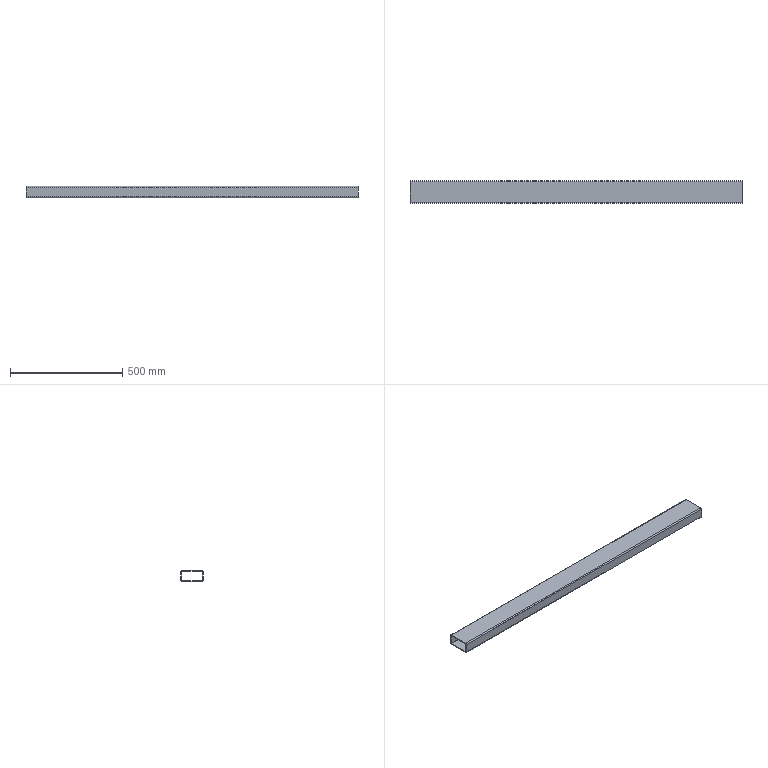Part | SolidWorks | features BaseBody 1 | 1 solid | 18 faces | box 1480 x 100 x 50 mm | volume 1650789 mm3 | plane 10 | cylinder 8 | commonest cylinder face diameters 2 x4 10 x4
STEP:
#1=CARTESIAN_POINT('',(-740.,45.,-25.));
#2=VERTEX_POINT('',#1);
#3=CARTESIAN_POINT('',(-740.,50.,-20.));
#4=VERTEX_POINT('',#3);
#5=CARTESIAN_POINT('',(-740.,45.,-20.));
#6=DIRECTION('',(1.,0.,0.));
#7=DIRECTION('',(0.,0.,-1.));
#8=AXIS2_PLACEMENT_3D('',#5,#6,#7);
#9=CIRCLE('',#8,5.);
#10=EDGE_CURVE('',#2,#4,#9,.T.);
#11=ORIENTED_EDGE('',*,*,#10,.T.);
#12=CARTESIAN_POINT('',(740.,50.,-20.));
#13=VERTEX_POINT('',#12);
#14=CARTESIAN_POINT('',(740.,50.,-20.));
#15=DIRECTION('',(-1.,0.,0.));
#16=VECTOR('',#15,1000.);
#17=LINE('',#14,#16);
#18=EDGE_CURVE('',#13,#4,#17,.T.);
#19=ORIENTED_EDGE('',*,*,#18,.F.);
#20=CARTESIAN_POINT('',(740.,45.,-25.));
#21=VERTEX_POINT('',#20);
#22=CARTESIAN_POINT('',(740.,45.,-20.));
#23=DIRECTION('',(1.,0.,0.));
#24=DIRECTION('',(0.,0.,-1.));
#25=AXIS2_PLACEMENT_3D('',#22,#23,#24);
#26=CIRCLE('',#25,5.);
#27=EDGE_CURVE('',#21,#13,#26,.T.);
#28=ORIENTED_EDGE('',*,*,#27,.F.);
#29=CARTESIAN_POINT('',(740.,45.,-25.));
#30=DIRECTION('',(-1.,0.,0.));
#31=VECTOR('',#30,1000.);
#32=LINE('',#29,#31);
#33=EDGE_CURVE('',#21,#2,#32,.T.);
#34=ORIENTED_EDGE('',*,*,#33,.T.);
#35=EDGE_LOOP('',(#11,#19,#28,#34));
#36=FACE_OUTER_BOUND('',#35,.T.);
#37=CARTESIAN_POINT('',(740.,45.,-20.));
#38=DIRECTION('',(-1.,0.,0.));
#39=DIRECTION('',(0.,0.,1.));
#40=AXIS2_PLACEMENT_3D('',#37,#38,#39);
#41=CYLINDRICAL_SURFACE('',#40,5.);
#42=ADVANCED_FACE('',(#36),#41,.T.);
#43=CARTESIAN_POINT('',(-740.,50.,20.));
#44=VERTEX_POINT('',#43);
#45=CARTESIAN_POINT('',(-740.,50.,-20.));
#46=DIRECTION('',(0.,0.,1.));
#47=VECTOR('',#46,1000.);
#48=LINE('',#45,#47);
#49=EDGE_CURVE('',#4,#44,#48,.T.);
#50=ORIENTED_EDGE('',*,*,#49,.T.);
#51=CARTESIAN_POINT('',(740.,50.,20.));
#52=VERTEX_POINT('',#51);
#53=CARTESIAN_POINT('',(740.,50.,20.));
#54=DIRECTION('',(-1.,0.,0.));
#55=VECTOR('',#54,1000.);
#56=LINE('',#53,#55);
#57=EDGE_CURVE('',#52,#44,#56,.T.);
#58=ORIENTED_EDGE('',*,*,#57,.F.);
#59=CARTESIAN_POINT('',(740.,50.,-20.));
#60=DIRECTION('',(0.,0.,1.));
#61=VECTOR('',#60,1000.);
#62=LINE('',#59,#61);
#63=EDGE_CURVE('',#13,#52,#62,.T.);
#64=ORIENTED_EDGE('',*,*,#63,.F.);
#65=ORIENTED_EDGE('',*,*,#18,.T.);
#66=EDGE_LOOP('',(#50,#58,#64,#65));
#67=FACE_OUTER_BOUND('',#66,.T.);
#68=CARTESIAN_POINT('',(740.,50.,-20.));
#69=DIRECTION('',(0.,-1.,0.));
#70=DIRECTION('',(0.,0.,-1.));
#71=AXIS2_PLACEMENT_3D('',#68,#69,#70);
#72=PLANE('',#71);
#73=ADVANCED_FACE('',(#67),#72,.F.);
#74=CARTESIAN_POINT('',(-740.,45.,25.));
#75=VERTEX_POINT('',#74);
#76=CARTESIAN_POINT('',(-740.,45.,20.));
#77=DIRECTION('',(1.,0.,0.));
#78=DIRECTION('',(0.,0.,-1.));
#79=AXIS2_PLACEMENT_3D('',#76,#77,#78);
#80=CIRCLE('',#79,5.);
#81=EDGE_CURVE('',#44,#75,#80,.T.);
#82=ORIENTED_EDGE('',*,*,#81,.T.);
#83=CARTESIAN_POINT('',(740.,45.,25.));
#84=VERTEX_POINT('',#83);
#85=CARTESIAN_POINT('',(740.,45.,25.));
#86=DIRECTION('',(-1.,0.,0.));
#87=VECTOR('',#86,1000.);
#88=LINE('',#85,#87);
#89=EDGE_CURVE('',#84,#75,#88,.T.);
#90=ORIENTED_EDGE('',*,*,#89,.F.);
#91=CARTESIAN_POINT('',(740.,45.,20.));
#92=DIRECTION('',(1.,0.,0.));
#93=DIRECTION('',(0.,0.,-1.));
#94=AXIS2_PLACEMENT_3D('',#91,#92,#93);
#95=CIRCLE('',#94,5.);
#96=EDGE_CURVE('',#52,#84,#95,.T.);
#97=ORIENTED_EDGE('',*,*,#96,.F.);
#98=ORIENTED_EDGE('',*,*,#57,.T.);
#99=EDGE_LOOP('',(#82,#90,#97,#98));
#100=FACE_OUTER_BOUND('',#99,.T.);
#101=CARTESIAN_POINT('',(740.,45.,20.));
#102=DIRECTION('',(-1.,0.,0.));
#103=DIRECTION('',(0.,0.,1.));
#104=AXIS2_PLACEMENT_3D('',#101,#102,#103);
#105=CYLINDRICAL_SURFACE('',#104,5.);
#106=ADVANCED_FACE('',(#100),#105,.T.);
#107=CARTESIAN_POINT('',(-740.,-45.,25.));
#108=VERTEX_POINT('',#107);
#109=CARTESIAN_POINT('',(-740.,-45.,25.));
#110=DIRECTION('',(0.,-1.,0.));
#111=VECTOR('',#110,1000.);
#112=LINE('',#109,#111);
#113=EDGE_CURVE('',#75,#108,#112,.T.);
#114=ORIENTED_EDGE('',*,*,#113,.T.);
#115=CARTESIAN_POINT('',(740.,-45.,25.));
#116=VERTEX_POINT('',#115);
#117=CARTESIAN_POINT('',(740.,-45.,25.));
#118=DIRECTION('',(-1.,0.,0.));
#119=VECTOR('',#118,1000.);
#120=LINE('',#117,#119);
#121=EDGE_CURVE('',#116,#108,#120,.T.);
#122=ORIENTED_EDGE('',*,*,#121,.F.);
#123=CARTESIAN_POINT('',(740.,-45.,25.));
#124=DIRECTION('',(0.,-1.,0.));
#125=VECTOR('',#124,1000.);
#126=LINE('',#123,#125);
#127=EDGE_CURVE('',#84,#116,#126,.T.);
#128=ORIENTED_EDGE('',*,*,#127,.F.);
#129=ORIENTED_EDGE('',*,*,#89,.T.);
#130=EDGE_LOOP('',(#114,#122,#128,#129));
#131=FACE_OUTER_BOUND('',#130,.T.);
#132=CARTESIAN_POINT('',(740.,-45.,25.));
#133=DIRECTION('',(0.,0.,-1.));
#134=DIRECTION('',(0.,1.,0.));
#135=AXIS2_PLACEMENT_3D('',#132,#133,#134);
#136=PLANE('',#135);
#137=ADVANCED_FACE('',(#131),#136,.F.);
#138=CARTESIAN_POINT('',(-740.,-50.,20.));
#139=VERTEX_POINT('',#138);
#140=CARTESIAN_POINT('',(-740.,-45.,20.));
#141=DIRECTION('',(1.,0.,0.));
#142=DIRECTION('',(0.,0.,-1.));
#143=AXIS2_PLACEMENT_3D('',#140,#141,#142);
#144=CIRCLE('',#143,5.);
#145=EDGE_CURVE('',#108,#139,#144,.T.);
#146=ORIENTED_EDGE('',*,*,#145,.T.);
#147=CARTESIAN_POINT('',(740.,-50.,20.));
#148=VERTEX_POINT('',#147);
#149=CARTESIAN_POINT('',(740.,-50.,20.));
#150=DIRECTION('',(-1.,0.,0.));
#151=VECTOR('',#150,1000.);
#152=LINE('',#149,#151);
#153=EDGE_CURVE('',#148,#139,#152,.T.);
#154=ORIENTED_EDGE('',*,*,#153,.F.);
#155=CARTESIAN_POINT('',(740.,-45.,20.));
#156=DIRECTION('',(1.,0.,0.));
#157=DIRECTION('',(0.,0.,-1.));
#158=AXIS2_PLACEMENT_3D('',#155,#156,#157);
#159=CIRCLE('',#158,5.);
#160=EDGE_CURVE('',#116,#148,#159,.T.);
#161=ORIENTED_EDGE('',*,*,#160,.F.);
#162=ORIENTED_EDGE('',*,*,#121,.T.);
#163=EDGE_LOOP('',(#146,#154,#161,#162));
#164=FACE_OUTER_BOUND('',#163,.T.);
#165=CARTESIAN_POINT('',(740.,-45.,20.));
#166=DIRECTION('',(-1.,0.,0.));
#167=DIRECTION('',(0.,0.,1.));
#168=AXIS2_PLACEMENT_3D('',#165,#166,#167);
#169=CYLINDRICAL_SURFACE('',#168,5.);
#170=ADVANCED_FACE('',(#164),#169,.T.);
#171=CARTESIAN_POINT('',(-740.,-50.,-20.));
#172=VERTEX_POINT('',#171);
#173=CARTESIAN_POINT('',(-740.,-50.,20.));
#174=DIRECTION('',(0.,0.,-1.));
#175=VECTOR('',#174,1000.);
#176=LINE('',#173,#175);
#177=EDGE_CURVE('',#139,#172,#176,.T.);
#178=ORIENTED_EDGE('',*,*,#177,.T.);
#179=CARTESIAN_POINT('',(740.,-50.,-20.));
#180=VERTEX_POINT('',#179);
#181=CARTESIAN_POINT('',(740.,-50.,-20.));
#182=DIRECTION('',(-1.,0.,0.));
#183=VECTOR('',#182,1000.);
#184=LINE('',#181,#183);
#185=EDGE_CURVE('',#180,#172,#184,.T.);
#186=ORIENTED_EDGE('',*,*,#185,.F.);
#187=CARTESIAN_POINT('',(740.,-50.,20.));
#188=DIRECTION('',(0.,0.,-1.));
#189=VECTOR('',#188,1000.);
#190=LINE('',#187,#189);
#191=EDGE_CURVE('',#148,#180,#190,.T.);
#192=ORIENTED_EDGE('',*,*,#191,.F.);
#193=ORIENTED_EDGE('',*,*,#153,.T.);
#194=EDGE_LOOP('',(#178,#186,#192,#193));
#195=FACE_OUTER_BOUND('',#194,.T.);
#196=CARTESIAN_POINT('',(740.,-50.,20.));
#197=DIRECTION('',(0.,1.,0.));
#198=DIRECTION('',(0.,0.,1.));
#199=AXIS2_PLACEMENT_3D('',#196,#197,#198);
#200=PLANE('',#199);
#201=ADVANCED_FACE('',(#195),#200,.F.);
#202=CARTESIAN_POINT('',(-740.,-45.,-25.));
#203=VERTEX_POINT('',#202);
#204=CARTESIAN_POINT('',(-740.,-45.,-20.));
#205=DIRECTION('',(1.,0.,0.));
#206=DIRECTION('',(0.,0.,-1.));
#207=AXIS2_PLACEMENT_3D('',#204,#205,#206);
#208=CIRCLE('',#207,5.);
#209=EDGE_CURVE('',#172,#203,#208,.T.);
#210=ORIENTED_EDGE('',*,*,#209,.T.);
#211=CARTESIAN_POINT('',(740.,-45.,-25.));
#212=VERTEX_POINT('',#211);
#213=CARTESIAN_POINT('',(740.,-45.,-25.));
#214=DIRECTION('',(-1.,0.,0.));
#215=VECTOR('',#214,1000.);
#216=LINE('',#213,#215);
#217=EDGE_CURVE('',#212,#203,#216,.T.);
#218=ORIENTED_EDGE('',*,*,#217,.F.);
#219=CARTESIAN_POINT('',(740.,-45.,-20.));
#220=DIRECTION('',(1.,0.,0.));
#221=DIRECTION('',(0.,0.,-1.));
#222=AXIS2_PLACEMENT_3D('',#219,#220,#221);
#223=CIRCLE('',#222,5.);
#224=EDGE_CURVE('',#180,#212,#223,.T.);
#225=ORIENTED_EDGE('',*,*,#224,.F.);
#226=ORIENTED_EDGE('',*,*,#185,.T.);
#227=EDGE_LOOP('',(#210,#218,#225,#226));
#228=FACE_OUTER_BOUND('',#227,.T.);
#229=CARTESIAN_POINT('',(740.,-45.,-20.));
#230=DIRECTION('',(-1.,0.,0.));
#231=DIRECTION('',(0.,0.,1.));
#232=AXIS2_PLACEMENT_3D('',#229,#230,#231);
#233=CYLINDRICAL_SURFACE('',#232,5.);
#234=ADVANCED_FACE('',(#228),#233,.T.);
#235=CARTESIAN_POINT('',(-740.,46.,20.));
#236=VERTEX_POINT('',#235);
#237=CARTESIAN_POINT('',(-740.,45.,21.));
#238=VERTEX_POINT('',#237);
#239=CARTESIAN_POINT('',(-740.,45.,20.));
#240=DIRECTION('',(1.,0.,0.));
#241=DIRECTION('',(0.,0.,-1.));
#242=AXIS2_PLACEMENT_3D('',#239,#240,#241);
#243=CIRCLE('',#242,1.);
#244=EDGE_CURVE('',#236,#238,#243,.T.);
#245=ORIENTED_EDGE('',*,*,#244,.F.);
#246=CARTESIAN_POINT('',(740.,46.,20.));
#247=VERTEX_POINT('',#246);
#248=CARTESIAN_POINT('',(740.,46.,20.));
#249=DIRECTION('',(-1.,0.,0.));
#250=VECTOR('',#249,1000.);
#251=LINE('',#248,#250);
#252=EDGE_CURVE('',#247,#236,#251,.T.);
#253=ORIENTED_EDGE('',*,*,#252,.F.);
#254=CARTESIAN_POINT('',(740.,45.,21.));
#255=VERTEX_POINT('',#254);
#256=CARTESIAN_POINT('',(740.,45.,20.));
#257=DIRECTION('',(1.,0.,0.));
#258=DIRECTION('',(0.,0.,-1.));
#259=AXIS2_PLACEMENT_3D('',#256,#257,#258);
#260=CIRCLE('',#259,1.);
#261=EDGE_CURVE('',#247,#255,#260,.T.);
#262=ORIENTED_EDGE('',*,*,#261,.T.);
#263=CARTESIAN_POINT('',(740.,45.,21.));
#264=DIRECTION('',(-1.,0.,0.));
#265=VECTOR('',#264,1000.);
#266=LINE('',#263,#265);
#267=EDGE_CURVE('',#255,#238,#266,.T.);
#268=ORIENTED_EDGE('',*,*,#267,.T.);
#269=EDGE_LOOP('',(#245,#253,#262,#268));
#270=FACE_OUTER_BOUND('',#269,.T.);
#271=CARTESIAN_POINT('',(740.,45.,20.));
#272=DIRECTION('',(-1.,0.,0.));
#273=DIRECTION('',(0.,0.,1.));
#274=AXIS2_PLACEMENT_3D('',#271,#272,#273);
#275=CYLINDRICAL_SURFACE('',#274,1.);
#276=ADVANCED_FACE('',(#270),#275,.F.);
#277=CARTESIAN_POINT('',(-740.,46.,-20.));
#278=VERTEX_POINT('',#277);
#279=CARTESIAN_POINT('',(-740.,46.,-20.));
#280=DIRECTION('',(0.,0.,1.));
#281=VECTOR('',#280,1000.);
#282=LINE('',#279,#281);
#283=EDGE_CURVE('',#278,#236,#282,.T.);
#284=ORIENTED_EDGE('',*,*,#283,.F.);
#285=CARTESIAN_POINT('',(740.,46.,-20.));
#286=VERTEX_POINT('',#285);
#287=CARTESIAN_POINT('',(740.,46.,-20.));
#288=DIRECTION('',(-1.,0.,0.));
#289=VECTOR('',#288,1000.);
#290=LINE('',#287,#289);
#291=EDGE_CURVE('',#286,#278,#290,.T.);
#292=ORIENTED_EDGE('',*,*,#291,.F.);
#293=CARTESIAN_POINT('',(740.,46.,-20.));
#294=DIRECTION('',(0.,0.,1.));
#295=VECTOR('',#294,1000.);
#296=LINE('',#293,#295);
#297=EDGE_CURVE('',#286,#247,#296,.T.);
#298=ORIENTED_EDGE('',*,*,#297,.T.);
#299=ORIENTED_EDGE('',*,*,#252,.T.);
#300=EDGE_LOOP('',(#284,#292,#298,#299));
#301=FACE_OUTER_BOUND('',#300,.T.);
#302=CARTESIAN_POINT('',(740.,46.,-20.));
#303=DIRECTION('',(0.,-1.,0.));
#304=DIRECTION('',(0.,0.,-1.));
#305=AXIS2_PLACEMENT_3D('',#302,#303,#304);
#306=PLANE('',#305);
#307=ADVANCED_FACE('',(#301),#306,.T.);
#308=CARTESIAN_POINT('',(-740.,45.,-21.));
#309=VERTEX_POINT('',#308);
#310=CARTESIAN_POINT('',(-740.,45.,-20.));
#311=DIRECTION('',(1.,0.,0.));
#312=DIRECTION('',(0.,0.,-1.));
#313=AXIS2_PLACEMENT_3D('',#310,#311,#312);
#314=CIRCLE('',#313,1.);
#315=EDGE_CURVE('',#309,#278,#314,.T.);
#316=ORIENTED_EDGE('',*,*,#315,.F.);
#317=CARTESIAN_POINT('',(740.,45.,-21.));
#318=VERTEX_POINT('',#317);
#319=CARTESIAN_POINT('',(740.,45.,-21.));
#320=DIRECTION('',(-1.,0.,0.));
#321=VECTOR('',#320,1000.);
#322=LINE('',#319,#321);
#323=EDGE_CURVE('',#318,#309,#322,.T.);
#324=ORIENTED_EDGE('',*,*,#323,.F.);
#325=CARTESIAN_POINT('',(740.,45.,-20.));
#326=DIRECTION('',(1.,0.,0.));
#327=DIRECTION('',(0.,0.,-1.));
#328=AXIS2_PLACEMENT_3D('',#325,#326,#327);
#329=CIRCLE('',#328,1.);
#330=EDGE_CURVE('',#318,#286,#329,.T.);
#331=ORIENTED_EDGE('',*,*,#330,.T.);
#332=ORIENTED_EDGE('',*,*,#291,.T.);
#333=EDGE_LOOP('',(#316,#324,#331,#332));
#334=FACE_OUTER_BOUND('',#333,.T.);
#335=CARTESIAN_POINT('',(740.,45.,-20.));
#336=DIRECTION('',(-1.,0.,0.));
#337=DIRECTION('',(0.,0.,1.));
#338=AXIS2_PLACEMENT_3D('',#335,#336,#337);
#339=CYLINDRICAL_SURFACE('',#338,1.);
#340=ADVANCED_FACE('',(#334),#339,.F.);
#341=CARTESIAN_POINT('',(-740.,-45.,-21.));
#342=VERTEX_POINT('',#341);
#343=CARTESIAN_POINT('',(-740.,45.,-21.));
#344=DIRECTION('',(0.,1.,0.));
#345=VECTOR('',#344,1000.);
#346=LINE('',#343,#345);
#347=EDGE_CURVE('',#342,#309,#346,.T.);
#348=ORIENTED_EDGE('',*,*,#347,.F.);
#349=CARTESIAN_POINT('',(740.,-45.,-21.));
#350=VERTEX_POINT('',#349);
#351=CARTESIAN_POINT('',(740.,-45.,-21.));
#352=DIRECTION('',(-1.,0.,0.));
#353=VECTOR('',#352,1000.);
#354=LINE('',#351,#353);
#355=EDGE_CURVE('',#350,#342,#354,.T.);
#356=ORIENTED_EDGE('',*,*,#355,.F.);
#357=CARTESIAN_POINT('',(740.,45.,-21.));
#358=DIRECTION('',(0.,1.,0.));
#359=VECTOR('',#358,1000.);
#360=LINE('',#357,#359);
#361=EDGE_CURVE('',#350,#318,#360,.T.);
#362=ORIENTED_EDGE('',*,*,#361,.T.);
#363=ORIENTED_EDGE('',*,*,#323,.T.);
#364=EDGE_LOOP('',(#348,#356,#362,#363));
#365=FACE_OUTER_BOUND('',#364,.T.);
#366=CARTESIAN_POINT('',(740.,45.,-21.));
#367=DIRECTION('',(0.,0.,1.));
#368=DIRECTION('',(1.,0.,0.));
#369=AXIS2_PLACEMENT_3D('',#366,#367,#368);
#370=PLANE('',#369);
#371=ADVANCED_FACE('',(#365),#370,.T.);
#372=CARTESIAN_POINT('',(-740.,-46.,-20.));
#373=VERTEX_POINT('',#372);
#374=CARTESIAN_POINT('',(-740.,-45.,-20.));
#375=DIRECTION('',(1.,0.,0.));
#376=DIRECTION('',(0.,0.,-1.));
#377=AXIS2_PLACEMENT_3D('',#374,#375,#376);
#378=CIRCLE('',#377,1.);
#379=EDGE_CURVE('',#373,#342,#378,.T.);
#380=ORIENTED_EDGE('',*,*,#379,.F.);
#381=CARTESIAN_POINT('',(740.,-46.,-20.));
#382=VERTEX_POINT('',#381);
#383=CARTESIAN_POINT('',(740.,-46.,-20.));
#384=DIRECTION('',(-1.,0.,0.));
#385=VECTOR('',#384,1000.);
#386=LINE('',#383,#385);
#387=EDGE_CURVE('',#382,#373,#386,.T.);
#388=ORIENTED_EDGE('',*,*,#387,.F.);
#389=CARTESIAN_POINT('',(740.,-45.,-20.));
#390=DIRECTION('',(1.,0.,0.));
#391=DIRECTION('',(0.,0.,-1.));
#392=AXIS2_PLACEMENT_3D('',#389,#390,#391);
#393=CIRCLE('',#392,1.);
#394=EDGE_CURVE('',#382,#350,#393,.T.);
#395=ORIENTED_EDGE('',*,*,#394,.T.);
#396=ORIENTED_EDGE('',*,*,#355,.T.);
#397=EDGE_LOOP('',(#380,#388,#395,#396));
#398=FACE_OUTER_BOUND('',#397,.T.);
#399=CARTESIAN_POINT('',(740.,-45.,-20.));
#400=DIRECTION('',(-1.,0.,0.));
#401=DIRECTION('',(0.,0.,1.));
#402=AXIS2_PLACEMENT_3D('',#399,#400,#401);
#403=CYLINDRICAL_SURFACE('',#402,1.);
#404=ADVANCED_FACE('',(#398),#403,.F.);
#405=CARTESIAN_POINT('',(-740.,-46.,20.));
#406=VERTEX_POINT('',#405);
#407=CARTESIAN_POINT('',(-740.,-46.,20.));
#408=DIRECTION('',(0.,0.,-1.));
#409=VECTOR('',#408,1000.);
#410=LINE('',#407,#409);
#411=EDGE_CURVE('',#406,#373,#410,.T.);
#412=ORIENTED_EDGE('',*,*,#411,.F.);
#413=CARTESIAN_POINT('',(740.,-46.,20.));
#414=VERTEX_POINT('',#413);
#415=CARTESIAN_POINT('',(740.,-46.,20.));
#416=DIRECTION('',(-1.,0.,0.));
#417=VECTOR('',#416,1000.);
#418=LINE('',#415,#417);
#419=EDGE_CURVE('',#414,#406,#418,.T.);
#420=ORIENTED_EDGE('',*,*,#419,.F.);
#421=CARTESIAN_POINT('',(740.,-46.,20.));
#422=DIRECTION('',(0.,0.,-1.));
#423=VECTOR('',#422,1000.);
#424=LINE('',#421,#423);
#425=EDGE_CURVE('',#414,#382,#424,.T.);
#426=ORIENTED_EDGE('',*,*,#425,.T.);
#427=ORIENTED_EDGE('',*,*,#387,.T.);
#428=EDGE_LOOP('',(#412,#420,#426,#427));
#429=FACE_OUTER_BOUND('',#428,.T.);
#430=CARTESIAN_POINT('',(740.,-46.,20.));
#431=DIRECTION('',(0.,1.,0.));
#432=DIRECTION('',(0.,0.,1.));
#433=AXIS2_PLACEMENT_3D('',#430,#431,#432);
#434=PLANE('',#433);
#435=ADVANCED_FACE('',(#429),#434,.T.);
#436=CARTESIAN_POINT('',(-740.,-45.,21.));
#437=VERTEX_POINT('',#436);
#438=CARTESIAN_POINT('',(-740.,-45.,20.));
#439=DIRECTION('',(1.,0.,0.));
#440=DIRECTION('',(0.,0.,-1.));
#441=AXIS2_PLACEMENT_3D('',#438,#439,#440);
#442=CIRCLE('',#441,1.);
#443=EDGE_CURVE('',#437,#406,#442,.T.);
#444=ORIENTED_EDGE('',*,*,#443,.F.);
#445=CARTESIAN_POINT('',(740.,-45.,21.));
#446=VERTEX_POINT('',#445);
#447=CARTESIAN_POINT('',(740.,-45.,21.));
#448=DIRECTION('',(-1.,0.,0.));
#449=VECTOR('',#448,1000.);
#450=LINE('',#447,#449);
#451=EDGE_CURVE('',#446,#437,#450,.T.);
#452=ORIENTED_EDGE('',*,*,#451,.F.);
#453=CARTESIAN_POINT('',(740.,-45.,20.));
#454=DIRECTION('',(1.,0.,0.));
#455=DIRECTION('',(0.,0.,-1.));
#456=AXIS2_PLACEMENT_3D('',#453,#454,#455);
#457=CIRCLE('',#456,1.);
#458=EDGE_CURVE('',#446,#414,#457,.T.);
#459=ORIENTED_EDGE('',*,*,#458,.T.);
#460=ORIENTED_EDGE('',*,*,#419,.T.);
#461=EDGE_LOOP('',(#444,#452,#459,#460));
#462=FACE_OUTER_BOUND('',#461,.T.);
#463=CARTESIAN_POINT('',(740.,-45.,20.));
#464=DIRECTION('',(-1.,0.,0.));
#465=DIRECTION('',(0.,0.,1.));
#466=AXIS2_PLACEMENT_3D('',#463,#464,#465);
#467=CYLINDRICAL_SURFACE('',#466,1.);
#468=ADVANCED_FACE('',(#462),#467,.F.);
#469=CARTESIAN_POINT('',(-740.,-45.,21.));
#470=DIRECTION('',(0.,-1.,0.));
#471=VECTOR('',#470,1000.);
#472=LINE('',#469,#471);
#473=EDGE_CURVE('',#238,#437,#472,.T.);
#474=ORIENTED_EDGE('',*,*,#473,.F.);
#475=ORIENTED_EDGE('',*,*,#267,.F.);
#476=CARTESIAN_POINT('',(740.,-45.,21.));
#477=DIRECTION('',(0.,-1.,0.));
#478=VECTOR('',#477,1000.);
#479=LINE('',#476,#478);
#480=EDGE_CURVE('',#255,#446,#479,.T.);
#481=ORIENTED_EDGE('',*,*,#480,.T.);
#482=ORIENTED_EDGE('',*,*,#451,.T.);
#483=EDGE_LOOP('',(#474,#475,#481,#482));
#484=FACE_OUTER_BOUND('',#483,.T.);
#485=CARTESIAN_POINT('',(740.,-45.,21.));
#486=DIRECTION('',(0.,0.,-1.));
#487=DIRECTION('',(0.,1.,0.));
#488=AXIS2_PLACEMENT_3D('',#485,#486,#487);
#489=PLANE('',#488);
#490=ADVANCED_FACE('',(#484),#489,.T.);
#491=CARTESIAN_POINT('',(-740.,45.,-25.));
#492=DIRECTION('',(0.,1.,0.));
#493=VECTOR('',#492,1000.);
#494=LINE('',#491,#493);
#495=EDGE_CURVE('',#203,#2,#494,.T.);
#496=ORIENTED_EDGE('',*,*,#495,.T.);
#497=ORIENTED_EDGE('',*,*,#33,.F.);
#498=CARTESIAN_POINT('',(740.,45.,-25.));
#499=DIRECTION('',(0.,1.,0.));
#500=VECTOR('',#499,1000.);
#501=LINE('',#498,#500);
#502=EDGE_CURVE('',#212,#21,#501,.T.);
#503=ORIENTED_EDGE('',*,*,#502,.F.);
#504=ORIENTED_EDGE('',*,*,#217,.T.);
#505=EDGE_LOOP('',(#496,#497,#503,#504));
#506=FACE_OUTER_BOUND('',#505,.T.);
#507=CARTESIAN_POINT('',(740.,45.,-25.));
#508=DIRECTION('',(0.,0.,1.));
#509=DIRECTION('',(1.,0.,0.));
#510=AXIS2_PLACEMENT_3D('',#507,#508,#509);
#511=PLANE('',#510);
#512=ADVANCED_FACE('',(#506),#511,.F.);
#513=ORIENTED_EDGE('',*,*,#261,.F.);
#514=ORIENTED_EDGE('',*,*,#297,.F.);
#515=ORIENTED_EDGE('',*,*,#330,.F.);
#516=ORIENTED_EDGE('',*,*,#361,.F.);
#517=ORIENTED_EDGE('',*,*,#394,.F.);
#518=ORIENTED_EDGE('',*,*,#425,.F.);
#519=ORIENTED_EDGE('',*,*,#458,.F.);
#520=ORIENTED_EDGE('',*,*,#480,.F.);
#521=EDGE_LOOP('',(#513,#514,#515,#516,#517,#518,#519,#520));
#522=FACE_BOUND('',#521,.T.);
#523=ORIENTED_EDGE('',*,*,#27,.T.);
#524=ORIENTED_EDGE('',*,*,#63,.T.);
#525=ORIENTED_EDGE('',*,*,#96,.T.);
#526=ORIENTED_EDGE('',*,*,#127,.T.);
#527=ORIENTED_EDGE('',*,*,#160,.T.);
#528=ORIENTED_EDGE('',*,*,#191,.T.);
#529=ORIENTED_EDGE('',*,*,#224,.T.);
#530=ORIENTED_EDGE('',*,*,#502,.T.);
#531=EDGE_LOOP('',(#523,#524,#525,#526,#527,#528,#529,#530));
#532=FACE_OUTER_BOUND('',#531,.T.);
#533=CARTESIAN_POINT('',(740.,45.,-20.));
#534=DIRECTION('',(1.,0.,0.));
#535=DIRECTION('',(0.,0.,-1.));
#536=AXIS2_PLACEMENT_3D('',#533,#534,#535);
#537=PLANE('',#536);
#538=ADVANCED_FACE('',(#522,#532),#537,.T.);
#539=ORIENTED_EDGE('',*,*,#244,.T.);
#540=ORIENTED_EDGE('',*,*,#473,.T.);
#541=ORIENTED_EDGE('',*,*,#443,.T.);
#542=ORIENTED_EDGE('',*,*,#411,.T.);
#543=ORIENTED_EDGE('',*,*,#379,.T.);
#544=ORIENTED_EDGE('',*,*,#347,.T.);
#545=ORIENTED_EDGE('',*,*,#315,.T.);
#546=ORIENTED_EDGE('',*,*,#283,.T.);
#547=EDGE_LOOP('',(#539,#540,#541,#542,#543,#544,#545,#546));
#548=FACE_BOUND('',#547,.T.);
#549=ORIENTED_EDGE('',*,*,#10,.F.);
#550=ORIENTED_EDGE('',*,*,#495,.F.);
#551=ORIENTED_EDGE('',*,*,#209,.F.);
#552=ORIENTED_EDGE('',*,*,#177,.F.);
#553=ORIENTED_EDGE('',*,*,#145,.F.);
#554=ORIENTED_EDGE('',*,*,#113,.F.);
#555=ORIENTED_EDGE('',*,*,#81,.F.);
#556=ORIENTED_EDGE('',*,*,#49,.F.);
#557=EDGE_LOOP('',(#549,#550,#551,#552,#553,#554,#555,#556));
#558=FACE_OUTER_BOUND('',#557,.T.);
#559=CARTESIAN_POINT('',(-740.,45.,-20.));
#560=DIRECTION('',(1.,0.,0.));
#561=DIRECTION('',(0.,0.,-1.));
#562=AXIS2_PLACEMENT_3D('',#559,#560,#561);
#563=PLANE('',#562);
#564=ADVANCED_FACE('',(#548,#558),#563,.F.);
#565=CLOSED_SHELL('',(#42,#73,#106,#137,#170,#201,#234,#276,#307,#340,#371,#404,#435,#468,#490,#512,#538,#564));
#566=MANIFOLD_SOLID_BREP('',#565);
#567=CARTESIAN_POINT('',(0.,0.,0.));
#568=DIRECTION('',(0.,0.,1.));
#569=DIRECTION('',(1.,0.,0.));
#570=AXIS2_PLACEMENT_3D('',#567,#568,#569);
#571=(LENGTH_UNIT()NAMED_UNIT(*)SI_UNIT(.MILLI.,.METRE.));
#572=UNCERTAINTY_MEASURE_WITH_UNIT(LENGTH_MEASURE(0.00001),#571,'','');
#573=(NAMED_UNIT(*)PLANE_ANGLE_UNIT()SI_UNIT($,.RADIAN.));
#574=(NAMED_UNIT(*)SI_UNIT($,.STERADIAN.)SOLID_ANGLE_UNIT());
#575=(GEOMETRIC_REPRESENTATION_CONTEXT(3)GLOBAL_UNCERTAINTY_ASSIGNED_CONTEXT((#572))GLOBAL_UNIT_ASSIGNED_CONTEXT((#571,#573,#574))REPRESENTATION_CONTEXT('',''));
#576=ADVANCED_BREP_SHAPE_REPRESENTATION('',(#566,#570),#575);